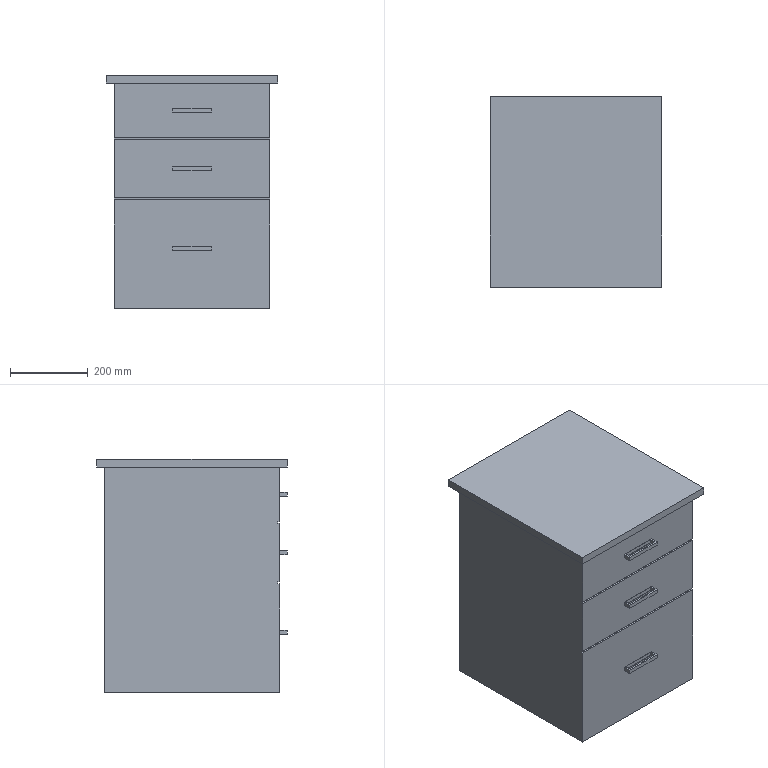Part | SolidWorks | features ICE 7, Extrusion 1 | 1 solid | 46 faces | box 440 x 490 x 600 mm | volume 108712401 mm3 | plane 46
STEP:
#1=CARTESIAN_POINT('',(400.,0.,280.));
#2=VERTEX_POINT('',#1);
#3=CARTESIAN_POINT('',(400.,0.,0.));
#4=VERTEX_POINT('',#3);
#5=CARTESIAN_POINT('',(400.,0.,600.));
#6=DIRECTION('',(0.,0.,-1.));
#7=VECTOR('',#6,1000.);
#8=LINE('',#5,#7);
#9=EDGE_CURVE('',#2,#4,#8,.T.);
#10=ORIENTED_EDGE('',*,*,#9,.F.);
#11=CARTESIAN_POINT('',(0.,0.,280.));
#12=VERTEX_POINT('',#11);
#13=CARTESIAN_POINT('',(0.,0.,280.));
#14=DIRECTION('',(1.,0.,0.));
#15=VECTOR('',#14,1000.);
#16=LINE('',#13,#15);
#17=EDGE_CURVE('',#12,#2,#16,.T.);
#18=ORIENTED_EDGE('',*,*,#17,.F.);
#19=CARTESIAN_POINT('',(0.,0.,0.));
#20=VERTEX_POINT('',#19);
#21=CARTESIAN_POINT('',(0.,0.,600.));
#22=DIRECTION('',(0.,0.,-1.));
#23=VECTOR('',#22,1000.);
#24=LINE('',#21,#23);
#25=EDGE_CURVE('',#12,#20,#24,.T.);
#26=ORIENTED_EDGE('',*,*,#25,.T.);
#27=CARTESIAN_POINT('',(0.,0.,0.));
#28=DIRECTION('',(1.,0.,0.));
#29=VECTOR('',#28,1000.);
#30=LINE('',#27,#29);
#31=EDGE_CURVE('',#20,#4,#30,.T.);
#32=ORIENTED_EDGE('',*,*,#31,.T.);
#33=EDGE_LOOP('',(#10,#18,#26,#32));
#34=FACE_OUTER_BOUND('',#33,.T.);
#35=CARTESIAN_POINT('',(150.,0.,160.));
#36=VERTEX_POINT('',#35);
#37=CARTESIAN_POINT('',(150.,0.,150.));
#38=VERTEX_POINT('',#37);
#39=CARTESIAN_POINT('',(150.,0.,150.));
#40=DIRECTION('',(0.,0.,-1.));
#41=VECTOR('',#40,1000.);
#42=LINE('',#39,#41);
#43=EDGE_CURVE('',#36,#38,#42,.T.);
#44=ORIENTED_EDGE('',*,*,#43,.F.);
#45=CARTESIAN_POINT('',(250.,0.,160.));
#46=VERTEX_POINT('',#45);
#47=CARTESIAN_POINT('',(150.,0.,160.));
#48=DIRECTION('',(-1.,0.,0.));
#49=VECTOR('',#48,1000.);
#50=LINE('',#47,#49);
#51=EDGE_CURVE('',#46,#36,#50,.T.);
#52=ORIENTED_EDGE('',*,*,#51,.F.);
#53=CARTESIAN_POINT('',(250.,0.,150.));
#54=VERTEX_POINT('',#53);
#55=CARTESIAN_POINT('',(250.,0.,150.));
#56=DIRECTION('',(0.,0.,1.));
#57=VECTOR('',#56,1000.);
#58=LINE('',#55,#57);
#59=EDGE_CURVE('',#54,#46,#58,.T.);
#60=ORIENTED_EDGE('',*,*,#59,.F.);
#61=CARTESIAN_POINT('',(150.,0.,150.));
#62=DIRECTION('',(1.,0.,0.));
#63=VECTOR('',#62,1000.);
#64=LINE('',#61,#63);
#65=EDGE_CURVE('',#38,#54,#64,.T.);
#66=ORIENTED_EDGE('',*,*,#65,.F.);
#67=EDGE_LOOP('',(#44,#52,#60,#66));
#68=FACE_BOUND('',#67,.T.);
#69=CARTESIAN_POINT('',(0.,0.,600.));
#70=DIRECTION('',(0.,1.,0.));
#71=DIRECTION('',(0.,0.,1.));
#72=AXIS2_PLACEMENT_3D('',#69,#70,#71);
#73=PLANE('',#72);
#74=ADVANCED_FACE('',(#34,#68),#73,.F.);
#75=CARTESIAN_POINT('',(0.,0.,435.));
#76=VERTEX_POINT('',#75);
#77=CARTESIAN_POINT('',(0.,0.,285.));
#78=VERTEX_POINT('',#77);
#79=CARTESIAN_POINT('',(0.,0.,600.));
#80=DIRECTION('',(0.,0.,-1.));
#81=VECTOR('',#80,1000.);
#82=LINE('',#79,#81);
#83=EDGE_CURVE('',#76,#78,#82,.T.);
#84=ORIENTED_EDGE('',*,*,#83,.T.);
#85=CARTESIAN_POINT('',(400.,0.,285.));
#86=VERTEX_POINT('',#85);
#87=CARTESIAN_POINT('',(0.,0.,285.));
#88=DIRECTION('',(-1.,0.,0.));
#89=VECTOR('',#88,1000.);
#90=LINE('',#87,#89);
#91=EDGE_CURVE('',#86,#78,#90,.T.);
#92=ORIENTED_EDGE('',*,*,#91,.F.);
#93=CARTESIAN_POINT('',(400.,0.,435.));
#94=VERTEX_POINT('',#93);
#95=CARTESIAN_POINT('',(400.,0.,600.));
#96=DIRECTION('',(0.,0.,-1.));
#97=VECTOR('',#96,1000.);
#98=LINE('',#95,#97);
#99=EDGE_CURVE('',#94,#86,#98,.T.);
#100=ORIENTED_EDGE('',*,*,#99,.F.);
#101=CARTESIAN_POINT('',(0.,0.,435.));
#102=DIRECTION('',(1.,0.,0.));
#103=VECTOR('',#102,1000.);
#104=LINE('',#101,#103);
#105=EDGE_CURVE('',#76,#94,#104,.T.);
#106=ORIENTED_EDGE('',*,*,#105,.F.);
#107=EDGE_LOOP('',(#84,#92,#100,#106));
#108=FACE_OUTER_BOUND('',#107,.T.);
#109=CARTESIAN_POINT('',(150.,0.,365.));
#110=VERTEX_POINT('',#109);
#111=CARTESIAN_POINT('',(150.,0.,355.));
#112=VERTEX_POINT('',#111);
#113=CARTESIAN_POINT('',(150.,0.,365.));
#114=DIRECTION('',(0.,0.,-1.));
#115=VECTOR('',#114,1000.);
#116=LINE('',#113,#115);
#117=EDGE_CURVE('',#110,#112,#116,.T.);
#118=ORIENTED_EDGE('',*,*,#117,.F.);
#119=CARTESIAN_POINT('',(250.,0.,365.));
#120=VERTEX_POINT('',#119);
#121=CARTESIAN_POINT('',(150.,0.,365.));
#122=DIRECTION('',(-1.,0.,0.));
#123=VECTOR('',#122,1000.);
#124=LINE('',#121,#123);
#125=EDGE_CURVE('',#120,#110,#124,.T.);
#126=ORIENTED_EDGE('',*,*,#125,.F.);
#127=CARTESIAN_POINT('',(250.,0.,355.));
#128=VERTEX_POINT('',#127);
#129=CARTESIAN_POINT('',(250.,0.,365.));
#130=DIRECTION('',(0.,0.,1.));
#131=VECTOR('',#130,1000.);
#132=LINE('',#129,#131);
#133=EDGE_CURVE('',#128,#120,#132,.T.);
#134=ORIENTED_EDGE('',*,*,#133,.F.);
#135=CARTESIAN_POINT('',(150.,0.,355.));
#136=DIRECTION('',(1.,0.,0.));
#137=VECTOR('',#136,1000.);
#138=LINE('',#135,#137);
#139=EDGE_CURVE('',#112,#128,#138,.T.);
#140=ORIENTED_EDGE('',*,*,#139,.F.);
#141=EDGE_LOOP('',(#118,#126,#134,#140));
#142=FACE_BOUND('',#141,.T.);
#143=CARTESIAN_POINT('',(0.,0.,600.));
#144=DIRECTION('',(0.,1.,0.));
#145=DIRECTION('',(0.,0.,1.));
#146=AXIS2_PLACEMENT_3D('',#143,#144,#145);
#147=PLANE('',#146);
#148=ADVANCED_FACE('',(#108,#142),#147,.F.);
#149=CARTESIAN_POINT('',(0.,0.,580.));
#150=VERTEX_POINT('',#149);
#151=CARTESIAN_POINT('',(0.,0.,440.));
#152=VERTEX_POINT('',#151);
#153=CARTESIAN_POINT('',(0.,0.,600.));
#154=DIRECTION('',(0.,0.,-1.));
#155=VECTOR('',#154,1000.);
#156=LINE('',#153,#155);
#157=EDGE_CURVE('',#150,#152,#156,.T.);
#158=ORIENTED_EDGE('',*,*,#157,.T.);
#159=CARTESIAN_POINT('',(400.,0.,440.));
#160=VERTEX_POINT('',#159);
#161=CARTESIAN_POINT('',(0.,0.,440.));
#162=DIRECTION('',(-1.,0.,0.));
#163=VECTOR('',#162,1000.);
#164=LINE('',#161,#163);
#165=EDGE_CURVE('',#160,#152,#164,.T.);
#166=ORIENTED_EDGE('',*,*,#165,.F.);
#167=CARTESIAN_POINT('',(400.,0.,580.));
#168=VERTEX_POINT('',#167);
#169=CARTESIAN_POINT('',(400.,0.,600.));
#170=DIRECTION('',(0.,0.,-1.));
#171=VECTOR('',#170,1000.);
#172=LINE('',#169,#171);
#173=EDGE_CURVE('',#168,#160,#172,.T.);
#174=ORIENTED_EDGE('',*,*,#173,.F.);
#175=CARTESIAN_POINT('',(0.,0.,580.));
#176=DIRECTION('',(1.,0.,0.));
#177=VECTOR('',#176,1000.);
#178=LINE('',#175,#177);
#179=EDGE_CURVE('',#150,#168,#178,.T.);
#180=ORIENTED_EDGE('',*,*,#179,.F.);
#181=EDGE_LOOP('',(#158,#166,#174,#180));
#182=FACE_OUTER_BOUND('',#181,.T.);
#183=CARTESIAN_POINT('',(150.,0.,515.));
#184=VERTEX_POINT('',#183);
#185=CARTESIAN_POINT('',(150.,0.,505.));
#186=VERTEX_POINT('',#185);
#187=CARTESIAN_POINT('',(150.,0.,515.));
#188=DIRECTION('',(0.,0.,-1.));
#189=VECTOR('',#188,1000.);
#190=LINE('',#187,#189);
#191=EDGE_CURVE('',#184,#186,#190,.T.);
#192=ORIENTED_EDGE('',*,*,#191,.F.);
#193=CARTESIAN_POINT('',(250.,0.,515.));
#194=VERTEX_POINT('',#193);
#195=CARTESIAN_POINT('',(150.,0.,515.));
#196=DIRECTION('',(-1.,0.,0.));
#197=VECTOR('',#196,1000.);
#198=LINE('',#195,#197);
#199=EDGE_CURVE('',#194,#184,#198,.T.);
#200=ORIENTED_EDGE('',*,*,#199,.F.);
#201=CARTESIAN_POINT('',(250.,0.,505.));
#202=VERTEX_POINT('',#201);
#203=CARTESIAN_POINT('',(250.,0.,515.));
#204=DIRECTION('',(0.,0.,1.));
#205=VECTOR('',#204,1000.);
#206=LINE('',#203,#205);
#207=EDGE_CURVE('',#202,#194,#206,.T.);
#208=ORIENTED_EDGE('',*,*,#207,.F.);
#209=CARTESIAN_POINT('',(150.,0.,505.));
#210=DIRECTION('',(1.,0.,0.));
#211=VECTOR('',#210,1000.);
#212=LINE('',#209,#211);
#213=EDGE_CURVE('',#186,#202,#212,.T.);
#214=ORIENTED_EDGE('',*,*,#213,.F.);
#215=EDGE_LOOP('',(#192,#200,#208,#214));
#216=FACE_BOUND('',#215,.T.);
#217=CARTESIAN_POINT('',(0.,0.,600.));
#218=DIRECTION('',(0.,1.,0.));
#219=DIRECTION('',(0.,0.,1.));
#220=AXIS2_PLACEMENT_3D('',#217,#218,#219);
#221=PLANE('',#220);
#222=ADVANCED_FACE('',(#182,#216),#221,.F.);
#223=CARTESIAN_POINT('',(0.,5.,285.));
#224=VERTEX_POINT('',#223);
#225=CARTESIAN_POINT('',(0.,5.,280.));
#226=VERTEX_POINT('',#225);
#227=CARTESIAN_POINT('',(0.,5.,285.));
#228=DIRECTION('',(0.,0.,-1.));
#229=VECTOR('',#228,1000.);
#230=LINE('',#227,#229);
#231=EDGE_CURVE('',#224,#226,#230,.T.);
#232=ORIENTED_EDGE('',*,*,#231,.F.);
#233=CARTESIAN_POINT('',(0.,5.,285.));
#234=DIRECTION('',(0.,-1.,0.));
#235=VECTOR('',#234,1000.);
#236=LINE('',#233,#235);
#237=EDGE_CURVE('',#224,#78,#236,.T.);
#238=ORIENTED_EDGE('',*,*,#237,.T.);
#239=ORIENTED_EDGE('',*,*,#83,.F.);
#240=CARTESIAN_POINT('',(0.,5.,435.));
#241=VERTEX_POINT('',#240);
#242=CARTESIAN_POINT('',(0.,5.,435.));
#243=DIRECTION('',(0.,-1.,0.));
#244=VECTOR('',#243,1000.);
#245=LINE('',#242,#244);
#246=EDGE_CURVE('',#241,#76,#245,.T.);
#247=ORIENTED_EDGE('',*,*,#246,.F.);
#248=CARTESIAN_POINT('',(0.,5.,440.));
#249=VERTEX_POINT('',#248);
#250=CARTESIAN_POINT('',(0.,5.,440.));
#251=DIRECTION('',(0.,0.,-1.));
#252=VECTOR('',#251,1000.);
#253=LINE('',#250,#252);
#254=EDGE_CURVE('',#249,#241,#253,.T.);
#255=ORIENTED_EDGE('',*,*,#254,.F.);
#256=CARTESIAN_POINT('',(0.,5.,440.));
#257=DIRECTION('',(0.,-1.,0.));
#258=VECTOR('',#257,1000.);
#259=LINE('',#256,#258);
#260=EDGE_CURVE('',#249,#152,#259,.T.);
#261=ORIENTED_EDGE('',*,*,#260,.T.);
#262=ORIENTED_EDGE('',*,*,#157,.F.);
#263=CARTESIAN_POINT('',(0.,450.,580.));
#264=VERTEX_POINT('',#263);
#265=CARTESIAN_POINT('',(0.,0.,580.));
#266=DIRECTION('',(0.,-1.,0.));
#267=VECTOR('',#266,1000.);
#268=LINE('',#265,#267);
#269=EDGE_CURVE('',#264,#150,#268,.T.);
#270=ORIENTED_EDGE('',*,*,#269,.F.);
#271=CARTESIAN_POINT('',(0.,450.,0.));
#272=VERTEX_POINT('',#271);
#273=CARTESIAN_POINT('',(0.,450.,600.));
#274=DIRECTION('',(0.,0.,-1.));
#275=VECTOR('',#274,1000.);
#276=LINE('',#273,#275);
#277=EDGE_CURVE('',#264,#272,#276,.T.);
#278=ORIENTED_EDGE('',*,*,#277,.T.);
#279=CARTESIAN_POINT('',(0.,0.,0.));
#280=DIRECTION('',(0.,-1.,0.));
#281=VECTOR('',#280,1000.);
#282=LINE('',#279,#281);
#283=EDGE_CURVE('',#272,#20,#282,.T.);
#284=ORIENTED_EDGE('',*,*,#283,.T.);
#285=ORIENTED_EDGE('',*,*,#25,.F.);
#286=CARTESIAN_POINT('',(0.,5.,280.));
#287=DIRECTION('',(0.,-1.,0.));
#288=VECTOR('',#287,1000.);
#289=LINE('',#286,#288);
#290=EDGE_CURVE('',#226,#12,#289,.T.);
#291=ORIENTED_EDGE('',*,*,#290,.F.);
#292=EDGE_LOOP('',(#232,#238,#239,#247,#255,#261,#262,#270,#278,#284,#285,#291));
#293=FACE_OUTER_BOUND('',#292,.T.);
#294=CARTESIAN_POINT('',(0.,0.,600.));
#295=DIRECTION('',(1.,0.,0.));
#296=DIRECTION('',(0.,0.,-1.));
#297=AXIS2_PLACEMENT_3D('',#294,#295,#296);
#298=PLANE('',#297);
#299=ADVANCED_FACE('',(#293),#298,.F.);
#300=ORIENTED_EDGE('',*,*,#99,.T.);
#301=CARTESIAN_POINT('',(400.,5.,285.));
#302=VERTEX_POINT('',#301);
#303=CARTESIAN_POINT('',(400.,5.,285.));
#304=DIRECTION('',(0.,-1.,0.));
#305=VECTOR('',#304,1000.);
#306=LINE('',#303,#305);
#307=EDGE_CURVE('',#302,#86,#306,.T.);
#308=ORIENTED_EDGE('',*,*,#307,.F.);
#309=CARTESIAN_POINT('',(400.,5.,280.));
#310=VERTEX_POINT('',#309);
#311=CARTESIAN_POINT('',(400.,5.,285.));
#312=DIRECTION('',(0.,0.,1.));
#313=VECTOR('',#312,1000.);
#314=LINE('',#311,#313);
#315=EDGE_CURVE('',#310,#302,#314,.T.);
#316=ORIENTED_EDGE('',*,*,#315,.F.);
#317=CARTESIAN_POINT('',(400.,5.,280.));
#318=DIRECTION('',(0.,-1.,0.));
#319=VECTOR('',#318,1000.);
#320=LINE('',#317,#319);
#321=EDGE_CURVE('',#310,#2,#320,.T.);
#322=ORIENTED_EDGE('',*,*,#321,.T.);
#323=ORIENTED_EDGE('',*,*,#9,.T.);
#324=CARTESIAN_POINT('',(400.,450.,0.));
#325=VERTEX_POINT('',#324);
#326=CARTESIAN_POINT('',(400.,0.,0.));
#327=DIRECTION('',(0.,1.,0.));
#328=VECTOR('',#327,1000.);
#329=LINE('',#326,#328);
#330=EDGE_CURVE('',#4,#325,#329,.T.);
#331=ORIENTED_EDGE('',*,*,#330,.T.);
#332=CARTESIAN_POINT('',(400.,450.,580.));
#333=VERTEX_POINT('',#332);
#334=CARTESIAN_POINT('',(400.,450.,600.));
#335=DIRECTION('',(0.,0.,-1.));
#336=VECTOR('',#335,1000.);
#337=LINE('',#334,#336);
#338=EDGE_CURVE('',#333,#325,#337,.T.);
#339=ORIENTED_EDGE('',*,*,#338,.F.);
#340=CARTESIAN_POINT('',(400.,0.,580.));
#341=DIRECTION('',(0.,1.,0.));
#342=VECTOR('',#341,1000.);
#343=LINE('',#340,#342);
#344=EDGE_CURVE('',#168,#333,#343,.T.);
#345=ORIENTED_EDGE('',*,*,#344,.F.);
#346=ORIENTED_EDGE('',*,*,#173,.T.);
#347=CARTESIAN_POINT('',(400.,5.,440.));
#348=VERTEX_POINT('',#347);
#349=CARTESIAN_POINT('',(400.,5.,440.));
#350=DIRECTION('',(0.,-1.,0.));
#351=VECTOR('',#350,1000.);
#352=LINE('',#349,#351);
#353=EDGE_CURVE('',#348,#160,#352,.T.);
#354=ORIENTED_EDGE('',*,*,#353,.F.);
#355=CARTESIAN_POINT('',(400.,5.,435.));
#356=VERTEX_POINT('',#355);
#357=CARTESIAN_POINT('',(400.,5.,440.));
#358=DIRECTION('',(0.,0.,1.));
#359=VECTOR('',#358,1000.);
#360=LINE('',#357,#359);
#361=EDGE_CURVE('',#356,#348,#360,.T.);
#362=ORIENTED_EDGE('',*,*,#361,.F.);
#363=CARTESIAN_POINT('',(400.,5.,435.));
#364=DIRECTION('',(0.,-1.,0.));
#365=VECTOR('',#364,1000.);
#366=LINE('',#363,#365);
#367=EDGE_CURVE('',#356,#94,#366,.T.);
#368=ORIENTED_EDGE('',*,*,#367,.T.);
#369=EDGE_LOOP('',(#300,#308,#316,#322,#323,#331,#339,#345,#346,#354,#362,#368));
#370=FACE_OUTER_BOUND('',#369,.T.);
#371=CARTESIAN_POINT('',(400.,0.,600.));
#372=DIRECTION('',(-1.,0.,0.));
#373=DIRECTION('',(0.,0.,1.));
#374=AXIS2_PLACEMENT_3D('',#371,#372,#373);
#375=PLANE('',#374);
#376=ADVANCED_FACE('',(#370),#375,.F.);
#377=CARTESIAN_POINT('',(0.,450.,580.));
#378=DIRECTION('',(-1.,0.,0.));
#379=VECTOR('',#378,1000.);
#380=LINE('',#377,#379);
#381=EDGE_CURVE('',#333,#264,#380,.T.);
#382=ORIENTED_EDGE('',*,*,#381,.F.);
#383=ORIENTED_EDGE('',*,*,#338,.T.);
#384=CARTESIAN_POINT('',(0.,450.,0.));
#385=DIRECTION('',(-1.,0.,0.));
#386=VECTOR('',#385,1000.);
#387=LINE('',#384,#386);
#388=EDGE_CURVE('',#325,#272,#387,.T.);
#389=ORIENTED_EDGE('',*,*,#388,.T.);
#390=ORIENTED_EDGE('',*,*,#277,.F.);
#391=EDGE_LOOP('',(#382,#383,#389,#390));
#392=FACE_OUTER_BOUND('',#391,.T.);
#393=CARTESIAN_POINT('',(0.,450.,600.));
#394=DIRECTION('',(0.,-1.,0.));
#395=DIRECTION('',(0.,0.,-1.));
#396=AXIS2_PLACEMENT_3D('',#393,#394,#395);
#397=PLANE('',#396);
#398=ADVANCED_FACE('',(#392),#397,.F.);
#399=ORIENTED_EDGE('',*,*,#283,.F.);
#400=ORIENTED_EDGE('',*,*,#388,.F.);
#401=ORIENTED_EDGE('',*,*,#330,.F.);
#402=ORIENTED_EDGE('',*,*,#31,.F.);
#403=EDGE_LOOP('',(#399,#400,#401,#402));
#404=FACE_OUTER_BOUND('',#403,.T.);
#405=CARTESIAN_POINT('',(0.,450.,0.));
#406=DIRECTION('',(0.,0.,-1.));
#407=DIRECTION('',(-1.,0.,0.));
#408=AXIS2_PLACEMENT_3D('',#405,#406,#407);
#409=PLANE('',#408);
#410=ADVANCED_FACE('',(#404),#409,.T.);
#411=CARTESIAN_POINT('',(-20.,470.,580.));
#412=VERTEX_POINT('',#411);
#413=CARTESIAN_POINT('',(-20.,-20.,580.));
#414=VERTEX_POINT('',#413);
#415=CARTESIAN_POINT('',(-20.,470.,580.));
#416=DIRECTION('',(0.,-1.,0.));
#417=VECTOR('',#416,1000.);
#418=LINE('',#415,#417);
#419=EDGE_CURVE('',#412,#414,#418,.T.);
#420=ORIENTED_EDGE('',*,*,#419,.F.);
#421=CARTESIAN_POINT('',(420.,470.,580.));
#422=VERTEX_POINT('',#421);
#423=CARTESIAN_POINT('',(-20.,470.,580.));
#424=DIRECTION('',(-1.,0.,0.));
#425=VECTOR('',#424,1000.);
#426=LINE('',#423,#425);
#427=EDGE_CURVE('',#422,#412,#426,.T.);
#428=ORIENTED_EDGE('',*,*,#427,.F.);
#429=CARTESIAN_POINT('',(420.,-20.,580.));
#430=VERTEX_POINT('',#429);
#431=CARTESIAN_POINT('',(420.,470.,580.));
#432=DIRECTION('',(0.,1.,0.));
#433=VECTOR('',#432,1000.);
#434=LINE('',#431,#433);
#435=EDGE_CURVE('',#430,#422,#434,.T.);
#436=ORIENTED_EDGE('',*,*,#435,.F.);
#437=CARTESIAN_POINT('',(-20.,-20.,580.));
#438=DIRECTION('',(1.,0.,0.));
#439=VECTOR('',#438,1000.);
#440=LINE('',#437,#439);
#441=EDGE_CURVE('',#414,#430,#440,.T.);
#442=ORIENTED_EDGE('',*,*,#441,.F.);
#443=EDGE_LOOP('',(#420,#428,#436,#442));
#444=FACE_OUTER_BOUND('',#443,.T.);
#445=ORIENTED_EDGE('',*,*,#381,.T.);
#446=ORIENTED_EDGE('',*,*,#269,.T.);
#447=ORIENTED_EDGE('',*,*,#179,.T.);
#448=ORIENTED_EDGE('',*,*,#344,.T.);
#449=EDGE_LOOP('',(#445,#446,#447,#448));
#450=FACE_BOUND('',#449,.T.);
#451=CARTESIAN_POINT('',(-20.,-20.,580.));
#452=DIRECTION('',(0.,0.,1.));
#453=DIRECTION('',(1.,0.,0.));
#454=AXIS2_PLACEMENT_3D('',#451,#452,#453);
#455=PLANE('',#454);
#456=ADVANCED_FACE('',(#444,#450),#455,.F.);
#457=CARTESIAN_POINT('',(-20.,470.,600.));
#458=VERTEX_POINT('',#457);
#459=CARTESIAN_POINT('',(-20.,-20.,600.));
#460=VERTEX_POINT('',#459);
#461=CARTESIAN_POINT('',(-20.,470.,600.));
#462=DIRECTION('',(0.,-1.,0.));
#463=VECTOR('',#462,1000.);
#464=LINE('',#461,#463);
#465=EDGE_CURVE('',#458,#460,#464,.T.);
#466=ORIENTED_EDGE('',*,*,#465,.F.);
#467=CARTESIAN_POINT('',(-20.,470.,580.));
#468=DIRECTION('',(0.,0.,1.));
#469=VECTOR('',#468,1000.);
#470=LINE('',#467,#469);
#471=EDGE_CURVE('',#412,#458,#470,.T.);
#472=ORIENTED_EDGE('',*,*,#471,.F.);
#473=ORIENTED_EDGE('',*,*,#419,.T.);
#474=CARTESIAN_POINT('',(-20.,-20.,580.));
#475=DIRECTION('',(0.,0.,1.));
#476=VECTOR('',#475,1000.);
#477=LINE('',#474,#476);
#478=EDGE_CURVE('',#414,#460,#477,.T.);
#479=ORIENTED_EDGE('',*,*,#478,.T.);
#480=EDGE_LOOP('',(#466,#472,#473,#479));
#481=FACE_OUTER_BOUND('',#480,.T.);
#482=CARTESIAN_POINT('',(-20.,470.,580.));
#483=DIRECTION('',(-1.,0.,0.));
#484=DIRECTION('',(0.,-1.,0.));
#485=AXIS2_PLACEMENT_3D('',#482,#483,#484);
#486=PLANE('',#485);
#487=ADVANCED_FACE('',(#481),#486,.T.);
#488=CARTESIAN_POINT('',(420.,470.,600.));
#489=VERTEX_POINT('',#488);
#490=CARTESIAN_POINT('',(-20.,470.,600.));
#491=DIRECTION('',(-1.,0.,0.));
#492=VECTOR('',#491,1000.);
#493=LINE('',#490,#492);
#494=EDGE_CURVE('',#489,#458,#493,.T.);
#495=ORIENTED_EDGE('',*,*,#494,.F.);
#496=CARTESIAN_POINT('',(420.,470.,580.));
#497=DIRECTION('',(0.,0.,1.));
#498=VECTOR('',#497,1000.);
#499=LINE('',#496,#498);
#500=EDGE_CURVE('',#422,#489,#499,.T.);
#501=ORIENTED_EDGE('',*,*,#500,.F.);
#502=ORIENTED_EDGE('',*,*,#427,.T.);
#503=ORIENTED_EDGE('',*,*,#471,.T.);
#504=EDGE_LOOP('',(#495,#501,#502,#503));
#505=FACE_OUTER_BOUND('',#504,.T.);
#506=CARTESIAN_POINT('',(-20.,470.,580.));
#507=DIRECTION('',(0.,1.,0.));
#508=DIRECTION('',(0.,0.,1.));
#509=AXIS2_PLACEMENT_3D('',#506,#507,#508);
#510=PLANE('',#509);
#511=ADVANCED_FACE('',(#505),#510,.T.);
#512=CARTESIAN_POINT('',(420.,-20.,600.));
#513=VERTEX_POINT('',#512);
#514=CARTESIAN_POINT('',(420.,470.,600.));
#515=DIRECTION('',(0.,1.,0.));
#516=VECTOR('',#515,1000.);
#517=LINE('',#514,#516);
#518=EDGE_CURVE('',#513,#489,#517,.T.);
#519=ORIENTED_EDGE('',*,*,#518,.F.);
#520=CARTESIAN_POINT('',(420.,-20.,580.));
#521=DIRECTION('',(0.,0.,1.));
#522=VECTOR('',#521,1000.);
#523=LINE('',#520,#522);
#524=EDGE_CURVE('',#430,#513,#523,.T.);
#525=ORIENTED_EDGE('',*,*,#524,.F.);
#526=ORIENTED_EDGE('',*,*,#435,.T.);
#527=ORIENTED_EDGE('',*,*,#500,.T.);
#528=EDGE_LOOP('',(#519,#525,#526,#527));
#529=FACE_OUTER_BOUND('',#528,.T.);
#530=CARTESIAN_POINT('',(420.,470.,580.));
#531=DIRECTION('',(1.,0.,0.));
#532=DIRECTION('',(0.,1.,0.));
#533=AXIS2_PLACEMENT_3D('',#530,#531,#532);
#534=PLANE('',#533);
#535=ADVANCED_FACE('',(#529),#534,.T.);
#536=CARTESIAN_POINT('',(-20.,-20.,600.));
#537=DIRECTION('',(1.,0.,0.));
#538=VECTOR('',#537,1000.);
#539=LINE('',#536,#538);
#540=EDGE_CURVE('',#460,#513,#539,.T.);
#541=ORIENTED_EDGE('',*,*,#540,.F.);
#542=ORIENTED_EDGE('',*,*,#478,.F.);
#543=ORIENTED_EDGE('',*,*,#441,.T.);
#544=ORIENTED_EDGE('',*,*,#524,.T.);
#545=EDGE_LOOP('',(#541,#542,#543,#544));
#546=FACE_OUTER_BOUND('',#545,.T.);
#547=CARTESIAN_POINT('',(-20.,-20.,580.));
#548=DIRECTION('',(0.,-1.,0.));
#549=DIRECTION('',(0.,0.,-1.));
#550=AXIS2_PLACEMENT_3D('',#547,#548,#549);
#551=PLANE('',#550);
#552=ADVANCED_FACE('',(#546),#551,.T.);
#553=ORIENTED_EDGE('',*,*,#465,.T.);
#554=ORIENTED_EDGE('',*,*,#540,.T.);
#555=ORIENTED_EDGE('',*,*,#518,.T.);
#556=ORIENTED_EDGE('',*,*,#494,.T.);
#557=EDGE_LOOP('',(#553,#554,#555,#556));
#558=FACE_OUTER_BOUND('',#557,.T.);
#559=CARTESIAN_POINT('',(0.,450.,600.));
#560=DIRECTION('',(0.,0.,-1.));
#561=DIRECTION('',(-1.,0.,0.));
#562=AXIS2_PLACEMENT_3D('',#559,#560,#561);
#563=PLANE('',#562);
#564=ADVANCED_FACE('',(#558),#563,.F.);
#565=ORIENTED_EDGE('',*,*,#165,.T.);
#566=ORIENTED_EDGE('',*,*,#260,.F.);
#567=CARTESIAN_POINT('',(0.,5.,440.));
#568=DIRECTION('',(-1.,0.,0.));
#569=VECTOR('',#568,1000.);
#570=LINE('',#567,#569);
#571=EDGE_CURVE('',#348,#249,#570,.T.);
#572=ORIENTED_EDGE('',*,*,#571,.F.);
#573=ORIENTED_EDGE('',*,*,#353,.T.);
#574=EDGE_LOOP('',(#565,#566,#572,#573));
#575=FACE_OUTER_BOUND('',#574,.T.);
#576=CARTESIAN_POINT('',(0.,5.,440.));
#577=DIRECTION('',(0.,0.,1.));
#578=DIRECTION('',(1.,0.,0.));
#579=AXIS2_PLACEMENT_3D('',#576,#577,#578);
#580=PLANE('',#579);
#581=ADVANCED_FACE('',(#575),#580,.F.);
#582=ORIENTED_EDGE('',*,*,#105,.T.);
#583=ORIENTED_EDGE('',*,*,#367,.F.);
#584=CARTESIAN_POINT('',(0.,5.,435.));
#585=DIRECTION('',(1.,0.,0.));
#586=VECTOR('',#585,1000.);
#587=LINE('',#584,#586);
#588=EDGE_CURVE('',#241,#356,#587,.T.);
#589=ORIENTED_EDGE('',*,*,#588,.F.);
#590=ORIENTED_EDGE('',*,*,#246,.T.);
#591=EDGE_LOOP('',(#582,#583,#589,#590));
#592=FACE_OUTER_BOUND('',#591,.T.);
#593=CARTESIAN_POINT('',(0.,5.,435.));
#594=DIRECTION('',(0.,0.,-1.));
#595=DIRECTION('',(-1.,0.,0.));
#596=AXIS2_PLACEMENT_3D('',#593,#594,#595);
#597=PLANE('',#596);
#598=ADVANCED_FACE('',(#592),#597,.F.);
#599=ORIENTED_EDGE('',*,*,#254,.T.);
#600=ORIENTED_EDGE('',*,*,#588,.T.);
#601=ORIENTED_EDGE('',*,*,#361,.T.);
#602=ORIENTED_EDGE('',*,*,#571,.T.);
#603=EDGE_LOOP('',(#599,#600,#601,#602));
#604=FACE_OUTER_BOUND('',#603,.T.);
#605=CARTESIAN_POINT('',(0.,5.,435.));
#606=DIRECTION('',(0.,-1.,0.));
#607=DIRECTION('',(0.,0.,-1.));
#608=AXIS2_PLACEMENT_3D('',#605,#606,#607);
#609=PLANE('',#608);
#610=ADVANCED_FACE('',(#604),#609,.T.);
#611=ORIENTED_EDGE('',*,*,#91,.T.);
#612=ORIENTED_EDGE('',*,*,#237,.F.);
#613=CARTESIAN_POINT('',(0.,5.,285.));
#614=DIRECTION('',(-1.,0.,0.));
#615=VECTOR('',#614,1000.);
#616=LINE('',#613,#615);
#617=EDGE_CURVE('',#302,#224,#616,.T.);
#618=ORIENTED_EDGE('',*,*,#617,.F.);
#619=ORIENTED_EDGE('',*,*,#307,.T.);
#620=EDGE_LOOP('',(#611,#612,#618,#619));
#621=FACE_OUTER_BOUND('',#620,.T.);
#622=CARTESIAN_POINT('',(0.,5.,285.));
#623=DIRECTION('',(0.,0.,1.));
#624=DIRECTION('',(1.,0.,0.));
#625=AXIS2_PLACEMENT_3D('',#622,#623,#624);
#626=PLANE('',#625);
#627=ADVANCED_FACE('',(#621),#626,.F.);
#628=ORIENTED_EDGE('',*,*,#17,.T.);
#629=ORIENTED_EDGE('',*,*,#321,.F.);
#630=CARTESIAN_POINT('',(0.,5.,280.));
#631=DIRECTION('',(1.,0.,0.));
#632=VECTOR('',#631,1000.);
#633=LINE('',#630,#632);
#634=EDGE_CURVE('',#226,#310,#633,.T.);
#635=ORIENTED_EDGE('',*,*,#634,.F.);
#636=ORIENTED_EDGE('',*,*,#290,.T.);
#637=EDGE_LOOP('',(#628,#629,#635,#636));
#638=FACE_OUTER_BOUND('',#637,.T.);
#639=CARTESIAN_POINT('',(0.,5.,280.));
#640=DIRECTION('',(0.,0.,-1.));
#641=DIRECTION('',(-1.,0.,0.));
#642=AXIS2_PLACEMENT_3D('',#639,#640,#641);
#643=PLANE('',#642);
#644=ADVANCED_FACE('',(#638),#643,.F.);
#645=ORIENTED_EDGE('',*,*,#231,.T.);
#646=ORIENTED_EDGE('',*,*,#634,.T.);
#647=ORIENTED_EDGE('',*,*,#315,.T.);
#648=ORIENTED_EDGE('',*,*,#617,.T.);
#649=EDGE_LOOP('',(#645,#646,#647,#648));
#650=FACE_OUTER_BOUND('',#649,.T.);
#651=CARTESIAN_POINT('',(0.,5.,280.));
#652=DIRECTION('',(0.,-1.,0.));
#653=DIRECTION('',(0.,0.,-1.));
#654=AXIS2_PLACEMENT_3D('',#651,#652,#653);
#655=PLANE('',#654);
#656=ADVANCED_FACE('',(#650),#655,.T.);
#657=ORIENTED_EDGE('',*,*,#191,.T.);
#658=CARTESIAN_POINT('',(150.,-20.,505.));
#659=VERTEX_POINT('',#658);
#660=CARTESIAN_POINT('',(150.,-20.,505.));
#661=DIRECTION('',(0.,1.,0.));
#662=VECTOR('',#661,1000.);
#663=LINE('',#660,#662);
#664=EDGE_CURVE('',#659,#186,#663,.T.);
#665=ORIENTED_EDGE('',*,*,#664,.F.);
#666=CARTESIAN_POINT('',(150.,-20.,515.));
#667=VERTEX_POINT('',#666);
#668=CARTESIAN_POINT('',(150.,-20.,515.));
#669=DIRECTION('',(0.,0.,-1.));
#670=VECTOR('',#669,1000.);
#671=LINE('',#668,#670);
#672=EDGE_CURVE('',#667,#659,#671,.T.);
#673=ORIENTED_EDGE('',*,*,#672,.F.);
#674=CARTESIAN_POINT('',(150.,-20.,515.));
#675=DIRECTION('',(0.,1.,0.));
#676=VECTOR('',#675,1000.);
#677=LINE('',#674,#676);
#678=EDGE_CURVE('',#667,#184,#677,.T.);
#679=ORIENTED_EDGE('',*,*,#678,.T.);
#680=EDGE_LOOP('',(#657,#665,#673,#679));
#681=FACE_OUTER_BOUND('',#680,.T.);
#682=CARTESIAN_POINT('',(150.,-20.,515.));
#683=DIRECTION('',(1.,0.,0.));
#684=DIRECTION('',(0.,0.,-1.));
#685=AXIS2_PLACEMENT_3D('',#682,#683,#684);
#686=PLANE('',#685);
#687=ADVANCED_FACE('',(#681),#686,.F.);
#688=CARTESIAN_POINT('',(245.,-0.3339,505.));
#689=VERTEX_POINT('',#688);
#690=CARTESIAN_POINT('',(155.,-0.3339,505.));
#691=VERTEX_POINT('',#690);
#692=CARTESIAN_POINT('',(150.,-0.3339,505.));
#693=DIRECTION('',(-1.,0.,0.));
#694=VECTOR('',#693,1000.);
#695=LINE('',#692,#694);
#696=EDGE_CURVE('',#689,#691,#695,.T.);
#697=ORIENTED_EDGE('',*,*,#696,.T.);
#698=CARTESIAN_POINT('',(155.,-15.,505.));
#699=VERTEX_POINT('',#698);
#700=CARTESIAN_POINT('',(155.,-20.,505.));
#701=DIRECTION('',(0.,-1.,0.));
#702=VECTOR('',#701,1000.);
#703=LINE('',#700,#702);
#704=EDGE_CURVE('',#691,#699,#703,.T.);
#705=ORIENTED_EDGE('',*,*,#704,.T.);
#706=CARTESIAN_POINT('',(245.,-15.,505.));
#707=VERTEX_POINT('',#706);
#708=CARTESIAN_POINT('',(150.,-15.,505.));
#709=DIRECTION('',(1.,0.,0.));
#710=VECTOR('',#709,1000.);
#711=LINE('',#708,#710);
#712=EDGE_CURVE('',#699,#707,#711,.T.);
#713=ORIENTED_EDGE('',*,*,#712,.T.);
#714=CARTESIAN_POINT('',(245.,-20.,505.));
#715=DIRECTION('',(0.,1.,0.));
#716=VECTOR('',#715,1000.);
#717=LINE('',#714,#716);
#718=EDGE_CURVE('',#707,#689,#717,.T.);
#719=ORIENTED_EDGE('',*,*,#718,.T.);
#720=EDGE_LOOP('',(#697,#705,#713,#719));
#721=FACE_BOUND('',#720,.T.);
#722=ORIENTED_EDGE('',*,*,#213,.T.);
#723=CARTESIAN_POINT('',(250.,-20.,505.));
#724=VERTEX_POINT('',#723);
#725=CARTESIAN_POINT('',(250.,-20.,505.));
#726=DIRECTION('',(0.,1.,0.));
#727=VECTOR('',#726,1000.);
#728=LINE('',#725,#727);
#729=EDGE_CURVE('',#724,#202,#728,.T.);
#730=ORIENTED_EDGE('',*,*,#729,.F.);
#731=CARTESIAN_POINT('',(150.,-20.,505.));
#732=DIRECTION('',(1.,0.,0.));
#733=VECTOR('',#732,1000.);
#734=LINE('',#731,#733);
#735=EDGE_CURVE('',#659,#724,#734,.T.);
#736=ORIENTED_EDGE('',*,*,#735,.F.);
#737=ORIENTED_EDGE('',*,*,#664,.T.);
#738=EDGE_LOOP('',(#722,#730,#736,#737));
#739=FACE_OUTER_BOUND('',#738,.T.);
#740=CARTESIAN_POINT('',(150.,-20.,505.));
#741=DIRECTION('',(0.,0.,1.));
#742=DIRECTION('',(1.,0.,0.));
#743=AXIS2_PLACEMENT_3D('',#740,#741,#742);
#744=PLANE('',#743);
#745=ADVANCED_FACE('',(#721,#739),#744,.F.);
#746=ORIENTED_EDGE('',*,*,#207,.T.);
#747=CARTESIAN_POINT('',(250.,-20.,515.));
#748=VERTEX_POINT('',#747);
#749=CARTESIAN_POINT('',(250.,-20.,515.));
#750=DIRECTION('',(0.,1.,0.));
#751=VECTOR('',#750,1000.);
#752=LINE('',#749,#751);
#753=EDGE_CURVE('',#748,#194,#752,.T.);
#754=ORIENTED_EDGE('',*,*,#753,.F.);
#755=CARTESIAN_POINT('',(250.,-20.,515.));
#756=DIRECTION('',(0.,0.,1.));
#757=VECTOR('',#756,1000.);
#758=LINE('',#755,#757);
#759=EDGE_CURVE('',#724,#748,#758,.T.);
#760=ORIENTED_EDGE('',*,*,#759,.F.);
#761=ORIENTED_EDGE('',*,*,#729,.T.);
#762=EDGE_LOOP('',(#746,#754,#760,#761));
#763=FACE_OUTER_BOUND('',#762,.T.);
#764=CARTESIAN_POINT('',(250.,-20.,515.));
#765=DIRECTION('',(-1.,0.,0.));
#766=DIRECTION('',(0.,0.,1.));
#767=AXIS2_PLACEMENT_3D('',#764,#765,#766);
#768=PLANE('',#767);
#769=ADVANCED_FACE('',(#763),#768,.F.);
#770=CARTESIAN_POINT('',(155.,-15.,515.));
#771=VERTEX_POINT('',#770);
#772=CARTESIAN_POINT('',(245.,-15.,515.));
#773=VERTEX_POINT('',#772);
#774=CARTESIAN_POINT('',(155.,-15.,515.));
#775=DIRECTION('',(1.,0.,0.));
#776=VECTOR('',#775,1000.);
#777=LINE('',#774,#776);
#778=EDGE_CURVE('',#771,#773,#777,.T.);
#779=ORIENTED_EDGE('',*,*,#778,.F.);
#780=CARTESIAN_POINT('',(155.,-0.3339,515.));
#781=VERTEX_POINT('',#780);
#782=CARTESIAN_POINT('',(155.,-0.3339,515.));
#783=DIRECTION('',(0.,-1.,0.));
#784=VECTOR('',#783,1000.);
#785=LINE('',#782,#784);
#786=EDGE_CURVE('',#781,#771,#785,.T.);
#787=ORIENTED_EDGE('',*,*,#786,.F.);
#788=CARTESIAN_POINT('',(245.,-0.3339,515.));
#789=VERTEX_POINT('',#788);
#790=CARTESIAN_POINT('',(155.,-0.3339,515.));
#791=DIRECTION('',(-1.,0.,0.));
#792=VECTOR('',#791,1000.);
#793=LINE('',#790,#792);
#794=EDGE_CURVE('',#789,#781,#793,.T.);
#795=ORIENTED_EDGE('',*,*,#794,.F.);
#796=CARTESIAN_POINT('',(245.,-0.3339,515.));
#797=DIRECTION('',(0.,1.,0.));
#798=VECTOR('',#797,1000.);
#799=LINE('',#796,#798);
#800=EDGE_CURVE('',#773,#789,#799,.T.);
#801=ORIENTED_EDGE('',*,*,#800,.F.);
#802=EDGE_LOOP('',(#779,#787,#795,#801));
#803=FACE_BOUND('',#802,.T.);
#804=ORIENTED_EDGE('',*,*,#199,.T.);
#805=ORIENTED_EDGE('',*,*,#678,.F.);
#806=CARTESIAN_POINT('',(150.,-20.,515.));
#807=DIRECTION('',(-1.,0.,0.));
#808=VECTOR('',#807,1000.);
#809=LINE('',#806,#808);
#810=EDGE_CURVE('',#748,#667,#809,.T.);
#811=ORIENTED_EDGE('',*,*,#810,.F.);
#812=ORIENTED_EDGE('',*,*,#753,.T.);
#813=EDGE_LOOP('',(#804,#805,#811,#812));
#814=FACE_OUTER_BOUND('',#813,.T.);
#815=CARTESIAN_POINT('',(150.,-20.,515.));
#816=DIRECTION('',(0.,0.,-1.));
#817=DIRECTION('',(-1.,0.,0.));
#818=AXIS2_PLACEMENT_3D('',#815,#816,#817);
#819=PLANE('',#818);
#820=ADVANCED_FACE('',(#803,#814),#819,.F.);
#821=ORIENTED_EDGE('',*,*,#672,.T.);
#822=ORIENTED_EDGE('',*,*,#735,.T.);
#823=ORIENTED_EDGE('',*,*,#759,.T.);
#824=ORIENTED_EDGE('',*,*,#810,.T.);
#825=EDGE_LOOP('',(#821,#822,#823,#824));
#826=FACE_OUTER_BOUND('',#825,.T.);
#827=CARTESIAN_POINT('',(150.,-20.,505.));
#828=DIRECTION('',(0.,-1.,0.));
#829=DIRECTION('',(0.,0.,-1.));
#830=AXIS2_PLACEMENT_3D('',#827,#828,#829);
#831=PLANE('',#830);
#832=ADVANCED_FACE('',(#826),#831,.T.);
#833=ORIENTED_EDGE('',*,*,#117,.T.);
#834=CARTESIAN_POINT('',(150.,-20.,355.));
#835=VERTEX_POINT('',#834);
#836=CARTESIAN_POINT('',(150.,-20.,355.));
#837=DIRECTION('',(0.,1.,0.));
#838=VECTOR('',#837,1000.);
#839=LINE('',#836,#838);
#840=EDGE_CURVE('',#835,#112,#839,.T.);
#841=ORIENTED_EDGE('',*,*,#840,.F.);
#842=CARTESIAN_POINT('',(150.,-20.,365.));
#843=VERTEX_POINT('',#842);
#844=CARTESIAN_POINT('',(150.,-20.,365.));
#845=DIRECTION('',(0.,0.,-1.));
#846=VECTOR('',#845,1000.);
#847=LINE('',#844,#846);
#848=EDGE_CURVE('',#843,#835,#847,.T.);
#849=ORIENTED_EDGE('',*,*,#848,.F.);
#850=CARTESIAN_POINT('',(150.,-20.,365.));
#851=DIRECTION('',(0.,1.,0.));
#852=VECTOR('',#851,1000.);
#853=LINE('',#850,#852);
#854=EDGE_CURVE('',#843,#110,#853,.T.);
#855=ORIENTED_EDGE('',*,*,#854,.T.);
#856=EDGE_LOOP('',(#833,#841,#849,#855));
#857=FACE_OUTER_BOUND('',#856,.T.);
#858=CARTESIAN_POINT('',(150.,-20.,365.));
#859=DIRECTION('',(1.,0.,0.));
#860=DIRECTION('',(0.,0.,-1.));
#861=AXIS2_PLACEMENT_3D('',#858,#859,#860);
#862=PLANE('',#861);
#863=ADVANCED_FACE('',(#857),#862,.F.);
#864=CARTESIAN_POINT('',(245.,-0.3339,355.));
#865=VERTEX_POINT('',#864);
#866=CARTESIAN_POINT('',(155.,-0.3339,355.));
#867=VERTEX_POINT('',#866);
#868=CARTESIAN_POINT('',(150.,-0.3339,355.));
#869=DIRECTION('',(-1.,0.,0.));
#870=VECTOR('',#869,1000.);
#871=LINE('',#868,#870);
#872=EDGE_CURVE('',#865,#867,#871,.T.);
#873=ORIENTED_EDGE('',*,*,#872,.T.);
#874=CARTESIAN_POINT('',(155.,-15.,355.));
#875=VERTEX_POINT('',#874);
#876=CARTESIAN_POINT('',(155.,-20.,355.));
#877=DIRECTION('',(0.,-1.,0.));
#878=VECTOR('',#877,1000.);
#879=LINE('',#876,#878);
#880=EDGE_CURVE('',#867,#875,#879,.T.);
#881=ORIENTED_EDGE('',*,*,#880,.T.);
#882=CARTESIAN_POINT('',(245.,-15.,355.));
#883=VERTEX_POINT('',#882);
#884=CARTESIAN_POINT('',(150.,-15.,355.));
#885=DIRECTION('',(1.,0.,0.));
#886=VECTOR('',#885,1000.);
#887=LINE('',#884,#886);
#888=EDGE_CURVE('',#875,#883,#887,.T.);
#889=ORIENTED_EDGE('',*,*,#888,.T.);
#890=CARTESIAN_POINT('',(245.,-20.,355.));
#891=DIRECTION('',(0.,1.,0.));
#892=VECTOR('',#891,1000.);
#893=LINE('',#890,#892);
#894=EDGE_CURVE('',#883,#865,#893,.T.);
#895=ORIENTED_EDGE('',*,*,#894,.T.);
#896=EDGE_LOOP('',(#873,#881,#889,#895));
#897=FACE_BOUND('',#896,.T.);
#898=ORIENTED_EDGE('',*,*,#139,.T.);
#899=CARTESIAN_POINT('',(250.,-20.,355.));
#900=VERTEX_POINT('',#899);
#901=CARTESIAN_POINT('',(250.,-20.,355.));
#902=DIRECTION('',(0.,1.,0.));
#903=VECTOR('',#902,1000.);
#904=LINE('',#901,#903);
#905=EDGE_CURVE('',#900,#128,#904,.T.);
#906=ORIENTED_EDGE('',*,*,#905,.F.);
#907=CARTESIAN_POINT('',(150.,-20.,355.));
#908=DIRECTION('',(1.,0.,0.));
#909=VECTOR('',#908,1000.);
#910=LINE('',#907,#909);
#911=EDGE_CURVE('',#835,#900,#910,.T.);
#912=ORIENTED_EDGE('',*,*,#911,.F.);
#913=ORIENTED_EDGE('',*,*,#840,.T.);
#914=EDGE_LOOP('',(#898,#906,#912,#913));
#915=FACE_OUTER_BOUND('',#914,.T.);
#916=CARTESIAN_POINT('',(150.,-20.,355.));
#917=DIRECTION('',(0.,0.,1.));
#918=DIRECTION('',(1.,0.,0.));
#919=AXIS2_PLACEMENT_3D('',#916,#917,#918);
#920=PLANE('',#919);
#921=ADVANCED_FACE('',(#897,#915),#920,.F.);
#922=ORIENTED_EDGE('',*,*,#133,.T.);
#923=CARTESIAN_POINT('',(250.,-20.,365.));
#924=VERTEX_POINT('',#923);
#925=CARTESIAN_POINT('',(250.,-20.,365.));
#926=DIRECTION('',(0.,1.,0.));
#927=VECTOR('',#926,1000.);
#928=LINE('',#925,#927);
#929=EDGE_CURVE('',#924,#120,#928,.T.);
#930=ORIENTED_EDGE('',*,*,#929,.F.);
#931=CARTESIAN_POINT('',(250.,-20.,365.));
#932=DIRECTION('',(0.,0.,1.));
#933=VECTOR('',#932,1000.);
#934=LINE('',#931,#933);
#935=EDGE_CURVE('',#900,#924,#934,.T.);
#936=ORIENTED_EDGE('',*,*,#935,.F.);
#937=ORIENTED_EDGE('',*,*,#905,.T.);
#938=EDGE_LOOP('',(#922,#930,#936,#937));
#939=FACE_OUTER_BOUND('',#938,.T.);
#940=CARTESIAN_POINT('',(250.,-20.,365.));
#941=DIRECTION('',(-1.,0.,0.));
#942=DIRECTION('',(0.,0.,1.));
#943=AXIS2_PLACEMENT_3D('',#940,#941,#942);
#944=PLANE('',#943);
#945=ADVANCED_FACE('',(#939),#944,.F.);
#946=CARTESIAN_POINT('',(245.,-15.,365.));
#947=VERTEX_POINT('',#946);
#948=CARTESIAN_POINT('',(155.,-15.,365.));
#949=VERTEX_POINT('',#948);
#950=CARTESIAN_POINT('',(150.,-15.,365.));
#951=DIRECTION('',(-1.,0.,0.));
#952=VECTOR('',#951,1000.);
#953=LINE('',#950,#952);
#954=EDGE_CURVE('',#947,#949,#953,.T.);
#955=ORIENTED_EDGE('',*,*,#954,.T.);
#956=CARTESIAN_POINT('',(155.,-0.3339,365.));
#957=VERTEX_POINT('',#956);
#958=CARTESIAN_POINT('',(155.,-20.,365.));
#959=DIRECTION('',(0.,1.,0.));
#960=VECTOR('',#959,1000.);
#961=LINE('',#958,#960);
#962=EDGE_CURVE('',#949,#957,#961,.T.);
#963=ORIENTED_EDGE('',*,*,#962,.T.);
#964=CARTESIAN_POINT('',(245.,-0.3339,365.));
#965=VERTEX_POINT('',#964);
#966=CARTESIAN_POINT('',(150.,-0.3339,365.));
#967=DIRECTION('',(1.,0.,0.));
#968=VECTOR('',#967,1000.);
#969=LINE('',#966,#968);
#970=EDGE_CURVE('',#957,#965,#969,.T.);
#971=ORIENTED_EDGE('',*,*,#970,.T.);
#972=CARTESIAN_POINT('',(245.,-20.,365.));
#973=DIRECTION('',(0.,-1.,0.));
#974=VECTOR('',#973,1000.);
#975=LINE('',#972,#974);
#976=EDGE_CURVE('',#965,#947,#975,.T.);
#977=ORIENTED_EDGE('',*,*,#976,.T.);
#978=EDGE_LOOP('',(#955,#963,#971,#977));
#979=FACE_BOUND('',#978,.T.);
#980=ORIENTED_EDGE('',*,*,#125,.T.);
#981=ORIENTED_EDGE('',*,*,#854,.F.);
#982=CARTESIAN_POINT('',(150.,-20.,365.));
#983=DIRECTION('',(-1.,0.,0.));
#984=VECTOR('',#983,1000.);
#985=LINE('',#982,#984);
#986=EDGE_CURVE('',#924,#843,#985,.T.);
#987=ORIENTED_EDGE('',*,*,#986,.F.);
#988=ORIENTED_EDGE('',*,*,#929,.T.);
#989=EDGE_LOOP('',(#980,#981,#987,#988));
#990=FACE_OUTER_BOUND('',#989,.T.);
#991=CARTESIAN_POINT('',(150.,-20.,365.));
#992=DIRECTION('',(0.,0.,-1.));
#993=DIRECTION('',(-1.,0.,0.));
#994=AXIS2_PLACEMENT_3D('',#991,#992,#993);
#995=PLANE('',#994);
#996=ADVANCED_FACE('',(#979,#990),#995,.F.);
#997=ORIENTED_EDGE('',*,*,#848,.T.);
#998=ORIENTED_EDGE('',*,*,#911,.T.);
#999=ORIENTED_EDGE('',*,*,#935,.T.);
#1000=ORIENTED_EDGE('',*,*,#986,.T.);
#1001=EDGE_LOOP('',(#997,#998,#999,#1000));
#1002=FACE_OUTER_BOUND('',#1001,.T.);
#1003=CARTESIAN_POINT('',(150.,-20.,355.));
#1004=DIRECTION('',(0.,-1.,0.));
#1005=DIRECTION('',(0.,0.,-1.));
#1006=AXIS2_PLACEMENT_3D('',#1003,#1004,#1005);
#1007=PLANE('',#1006);
#1008=ADVANCED_FACE('',(#1002),#1007,.T.);
#1009=ORIENTED_EDGE('',*,*,#43,.T.);
#1010=CARTESIAN_POINT('',(150.,-20.,150.));
#1011=VERTEX_POINT('',#1010);
#1012=CARTESIAN_POINT('',(150.,-20.,150.));
#1013=DIRECTION('',(0.,1.,0.));
#1014=VECTOR('',#1013,1000.);
#1015=LINE('',#1012,#1014);
#1016=EDGE_CURVE('',#1011,#38,#1015,.T.);
#1017=ORIENTED_EDGE('',*,*,#1016,.F.);
#1018=CARTESIAN_POINT('',(150.,-20.,160.));
#1019=VERTEX_POINT('',#1018);
#1020=CARTESIAN_POINT('',(150.,-20.,150.));
#1021=DIRECTION('',(0.,0.,-1.));
#1022=VECTOR('',#1021,1000.);
#1023=LINE('',#1020,#1022);
#1024=EDGE_CURVE('',#1019,#1011,#1023,.T.);
#1025=ORIENTED_EDGE('',*,*,#1024,.F.);
#1026=CARTESIAN_POINT('',(150.,-20.,160.));
#1027=DIRECTION('',(0.,1.,0.));
#1028=VECTOR('',#1027,1000.);
#1029=LINE('',#1026,#1028);
#1030=EDGE_CURVE('',#1019,#36,#1029,.T.);
#1031=ORIENTED_EDGE('',*,*,#1030,.T.);
#1032=EDGE_LOOP('',(#1009,#1017,#1025,#1031));
#1033=FACE_OUTER_BOUND('',#1032,.T.);
#1034=CARTESIAN_POINT('',(150.,-20.,150.));
#1035=DIRECTION('',(1.,0.,0.));
#1036=DIRECTION('',(0.,0.,-1.));
#1037=AXIS2_PLACEMENT_3D('',#1034,#1035,#1036);
#1038=PLANE('',#1037);
#1039=ADVANCED_FACE('',(#1033),#1038,.F.);
#1040=CARTESIAN_POINT('',(245.,-0.3339,150.));
#1041=VERTEX_POINT('',#1040);
#1042=CARTESIAN_POINT('',(155.,-0.3339,150.));
#1043=VERTEX_POINT('',#1042);
#1044=CARTESIAN_POINT('',(150.,-0.3339,150.));
#1045=DIRECTION('',(-1.,0.,0.));
#1046=VECTOR('',#1045,1000.);
#1047=LINE('',#1044,#1046);
#1048=EDGE_CURVE('',#1041,#1043,#1047,.T.);
#1049=ORIENTED_EDGE('',*,*,#1048,.T.);
#1050=CARTESIAN_POINT('',(155.,-15.,150.));
#1051=VERTEX_POINT('',#1050);
#1052=CARTESIAN_POINT('',(155.,-20.,150.));
#1053=DIRECTION('',(0.,-1.,0.));
#1054=VECTOR('',#1053,1000.);
#1055=LINE('',#1052,#1054);
#1056=EDGE_CURVE('',#1043,#1051,#1055,.T.);
#1057=ORIENTED_EDGE('',*,*,#1056,.T.);
#1058=CARTESIAN_POINT('',(245.,-15.,150.));
#1059=VERTEX_POINT('',#1058);
#1060=CARTESIAN_POINT('',(150.,-15.,150.));
#1061=DIRECTION('',(1.,0.,0.));
#1062=VECTOR('',#1061,1000.);
#1063=LINE('',#1060,#1062);
#1064=EDGE_CURVE('',#1051,#1059,#1063,.T.);
#1065=ORIENTED_EDGE('',*,*,#1064,.T.);
#1066=CARTESIAN_POINT('',(245.,-20.,150.));
#1067=DIRECTION('',(0.,1.,0.));
#1068=VECTOR('',#1067,1000.);
#1069=LINE('',#1066,#1068);
#1070=EDGE_CURVE('',#1059,#1041,#1069,.T.);
#1071=ORIENTED_EDGE('',*,*,#1070,.T.);
#1072=EDGE_LOOP('',(#1049,#1057,#1065,#1071));
#1073=FACE_BOUND('',#1072,.T.);
#1074=ORIENTED_EDGE('',*,*,#65,.T.);
#1075=CARTESIAN_POINT('',(250.,-20.,150.));
#1076=VERTEX_POINT('',#1075);
#1077=CARTESIAN_POINT('',(250.,-20.,150.));
#1078=DIRECTION('',(0.,1.,0.));
#1079=VECTOR('',#1078,1000.);
#1080=LINE('',#1077,#1079);
#1081=EDGE_CURVE('',#1076,#54,#1080,.T.);
#1082=ORIENTED_EDGE('',*,*,#1081,.F.);
#1083=CARTESIAN_POINT('',(150.,-20.,150.));
#1084=DIRECTION('',(1.,0.,0.));
#1085=VECTOR('',#1084,1000.);
#1086=LINE('',#1083,#1085);
#1087=EDGE_CURVE('',#1011,#1076,#1086,.T.);
#1088=ORIENTED_EDGE('',*,*,#1087,.F.);
#1089=ORIENTED_EDGE('',*,*,#1016,.T.);
#1090=EDGE_LOOP('',(#1074,#1082,#1088,#1089));
#1091=FACE_OUTER_BOUND('',#1090,.T.);
#1092=CARTESIAN_POINT('',(150.,-20.,150.));
#1093=DIRECTION('',(0.,0.,1.));
#1094=DIRECTION('',(1.,0.,0.));
#1095=AXIS2_PLACEMENT_3D('',#1092,#1093,#1094);
#1096=PLANE('',#1095);
#1097=ADVANCED_FACE('',(#1073,#1091),#1096,.F.);
#1098=ORIENTED_EDGE('',*,*,#59,.T.);
#1099=CARTESIAN_POINT('',(250.,-20.,160.));
#1100=VERTEX_POINT('',#1099);
#1101=CARTESIAN_POINT('',(250.,-20.,160.));
#1102=DIRECTION('',(0.,1.,0.));
#1103=VECTOR('',#1102,1000.);
#1104=LINE('',#1101,#1103);
#1105=EDGE_CURVE('',#1100,#46,#1104,.T.);
#1106=ORIENTED_EDGE('',*,*,#1105,.F.);
#1107=CARTESIAN_POINT('',(250.,-20.,150.));
#1108=DIRECTION('',(0.,0.,1.));
#1109=VECTOR('',#1108,1000.);
#1110=LINE('',#1107,#1109);
#1111=EDGE_CURVE('',#1076,#1100,#1110,.T.);
#1112=ORIENTED_EDGE('',*,*,#1111,.F.);
#1113=ORIENTED_EDGE('',*,*,#1081,.T.);
#1114=EDGE_LOOP('',(#1098,#1106,#1112,#1113));
#1115=FACE_OUTER_BOUND('',#1114,.T.);
#1116=CARTESIAN_POINT('',(250.,-20.,150.));
#1117=DIRECTION('',(-1.,0.,0.));
#1118=DIRECTION('',(0.,0.,1.));
#1119=AXIS2_PLACEMENT_3D('',#1116,#1117,#1118);
#1120=PLANE('',#1119);
#1121=ADVANCED_FACE('',(#1115),#1120,.F.);
#1122=CARTESIAN_POINT('',(245.,-15.,160.));
#1123=VERTEX_POINT('',#1122);
#1124=CARTESIAN_POINT('',(155.,-15.,160.));
#1125=VERTEX_POINT('',#1124);
#1126=CARTESIAN_POINT('',(150.,-15.,160.));
#1127=DIRECTION('',(-1.,0.,0.));
#1128=VECTOR('',#1127,1000.);
#1129=LINE('',#1126,#1128);
#1130=EDGE_CURVE('',#1123,#1125,#1129,.T.);
#1131=ORIENTED_EDGE('',*,*,#1130,.T.);
#1132=CARTESIAN_POINT('',(155.,-0.3339,160.));
#1133=VERTEX_POINT('',#1132);
#1134=CARTESIAN_POINT('',(155.,-20.,160.));
#1135=DIRECTION('',(0.,1.,0.));
#1136=VECTOR('',#1135,1000.);
#1137=LINE('',#1134,#1136);
#1138=EDGE_CURVE('',#1125,#1133,#1137,.T.);
#1139=ORIENTED_EDGE('',*,*,#1138,.T.);
#1140=CARTESIAN_POINT('',(245.,-0.3339,160.));
#1141=VERTEX_POINT('',#1140);
#1142=CARTESIAN_POINT('',(150.,-0.3339,160.));
#1143=DIRECTION('',(1.,0.,0.));
#1144=VECTOR('',#1143,1000.);
#1145=LINE('',#1142,#1144);
#1146=EDGE_CURVE('',#1133,#1141,#1145,.T.);
#1147=ORIENTED_EDGE('',*,*,#1146,.T.);
#1148=CARTESIAN_POINT('',(245.,-20.,160.));
#1149=DIRECTION('',(0.,-1.,0.));
#1150=VECTOR('',#1149,1000.);
#1151=LINE('',#1148,#1150);
#1152=EDGE_CURVE('',#1141,#1123,#1151,.T.);
#1153=ORIENTED_EDGE('',*,*,#1152,.T.);
#1154=EDGE_LOOP('',(#1131,#1139,#1147,#1153));
#1155=FACE_BOUND('',#1154,.T.);
#1156=ORIENTED_EDGE('',*,*,#51,.T.);
#1157=ORIENTED_EDGE('',*,*,#1030,.F.);
#1158=CARTESIAN_POINT('',(150.,-20.,160.));
#1159=DIRECTION('',(-1.,0.,0.));
#1160=VECTOR('',#1159,1000.);
#1161=LINE('',#1158,#1160);
#1162=EDGE_CURVE('',#1100,#1019,#1161,.T.);
#1163=ORIENTED_EDGE('',*,*,#1162,.F.);
#1164=ORIENTED_EDGE('',*,*,#1105,.T.);
#1165=EDGE_LOOP('',(#1156,#1157,#1163,#1164));
#1166=FACE_OUTER_BOUND('',#1165,.T.);
#1167=CARTESIAN_POINT('',(150.,-20.,160.));
#1168=DIRECTION('',(0.,0.,-1.));
#1169=DIRECTION('',(-1.,0.,0.));
#1170=AXIS2_PLACEMENT_3D('',#1167,#1168,#1169);
#1171=PLANE('',#1170);
#1172=ADVANCED_FACE('',(#1155,#1166),#1171,.F.);
#1173=ORIENTED_EDGE('',*,*,#1024,.T.);
#1174=ORIENTED_EDGE('',*,*,#1087,.T.);
#1175=ORIENTED_EDGE('',*,*,#1111,.T.);
#1176=ORIENTED_EDGE('',*,*,#1162,.T.);
#1177=EDGE_LOOP('',(#1173,#1174,#1175,#1176));
#1178=FACE_OUTER_BOUND('',#1177,.T.);
#1179=CARTESIAN_POINT('',(150.,-20.,160.));
#1180=DIRECTION('',(0.,1.,0.));
#1181=DIRECTION('',(0.,0.,1.));
#1182=AXIS2_PLACEMENT_3D('',#1179,#1180,#1181);
#1183=PLANE('',#1182);
#1184=ADVANCED_FACE('',(#1178),#1183,.F.);
#1185=CARTESIAN_POINT('',(155.,-15.,15.));
#1186=DIRECTION('',(0.,0.,1.));
#1187=VECTOR('',#1186,1000.);
#1188=LINE('',#1185,#1187);
#1189=EDGE_CURVE('',#1051,#1125,#1188,.T.);
#1190=ORIENTED_EDGE('',*,*,#1189,.T.);
#1191=ORIENTED_EDGE('',*,*,#1130,.F.);
#1192=CARTESIAN_POINT('',(245.,-15.,15.));
#1193=DIRECTION('',(0.,0.,1.));
#1194=VECTOR('',#1193,1000.);
#1195=LINE('',#1192,#1194);
#1196=EDGE_CURVE('',#1059,#1123,#1195,.T.);
#1197=ORIENTED_EDGE('',*,*,#1196,.F.);
#1198=ORIENTED_EDGE('',*,*,#1064,.F.);
#1199=EDGE_LOOP('',(#1190,#1191,#1197,#1198));
#1200=FACE_OUTER_BOUND('',#1199,.T.);
#1201=CARTESIAN_POINT('',(155.,-15.,15.));
#1202=DIRECTION('',(0.,-1.,0.));
#1203=DIRECTION('',(0.,0.,-1.));
#1204=AXIS2_PLACEMENT_3D('',#1201,#1202,#1203);
#1205=PLANE('',#1204);
#1206=ADVANCED_FACE('',(#1200),#1205,.F.);
#1207=ORIENTED_EDGE('',*,*,#1196,.T.);
#1208=ORIENTED_EDGE('',*,*,#1152,.F.);
#1209=CARTESIAN_POINT('',(245.,-0.3339,15.));
#1210=DIRECTION('',(0.,0.,1.));
#1211=VECTOR('',#1210,1000.);
#1212=LINE('',#1209,#1211);
#1213=EDGE_CURVE('',#1041,#1141,#1212,.T.);
#1214=ORIENTED_EDGE('',*,*,#1213,.F.);
#1215=ORIENTED_EDGE('',*,*,#1070,.F.);
#1216=EDGE_LOOP('',(#1207,#1208,#1214,#1215));
#1217=FACE_OUTER_BOUND('',#1216,.T.);
#1218=CARTESIAN_POINT('',(245.,-0.3339,15.));
#1219=DIRECTION('',(1.,0.,0.));
#1220=DIRECTION('',(0.,0.,-1.));
#1221=AXIS2_PLACEMENT_3D('',#1218,#1219,#1220);
#1222=PLANE('',#1221);
#1223=ADVANCED_FACE('',(#1217),#1222,.F.);
#1224=ORIENTED_EDGE('',*,*,#1213,.T.);
#1225=ORIENTED_EDGE('',*,*,#1146,.F.);
#1226=CARTESIAN_POINT('',(155.,-0.3339,15.));
#1227=DIRECTION('',(0.,0.,1.));
#1228=VECTOR('',#1227,1000.);
#1229=LINE('',#1226,#1228);
#1230=EDGE_CURVE('',#1043,#1133,#1229,.T.);
#1231=ORIENTED_EDGE('',*,*,#1230,.F.);
#1232=ORIENTED_EDGE('',*,*,#1048,.F.);
#1233=EDGE_LOOP('',(#1224,#1225,#1231,#1232));
#1234=FACE_OUTER_BOUND('',#1233,.T.);
#1235=CARTESIAN_POINT('',(155.,-0.3339,15.));
#1236=DIRECTION('',(0.,1.,0.));
#1237=DIRECTION('',(0.,0.,1.));
#1238=AXIS2_PLACEMENT_3D('',#1235,#1236,#1237);
#1239=PLANE('',#1238);
#1240=ADVANCED_FACE('',(#1234),#1239,.F.);
#1241=ORIENTED_EDGE('',*,*,#1230,.T.);
#1242=ORIENTED_EDGE('',*,*,#1138,.F.);
#1243=ORIENTED_EDGE('',*,*,#1189,.F.);
#1244=ORIENTED_EDGE('',*,*,#1056,.F.);
#1245=EDGE_LOOP('',(#1241,#1242,#1243,#1244));
#1246=FACE_OUTER_BOUND('',#1245,.T.);
#1247=CARTESIAN_POINT('',(155.,-0.3339,15.));
#1248=DIRECTION('',(-1.,0.,0.));
#1249=DIRECTION('',(0.,0.,1.));
#1250=AXIS2_PLACEMENT_3D('',#1247,#1248,#1249);
#1251=PLANE('',#1250);
#1252=ADVANCED_FACE('',(#1246),#1251,.F.);
#1253=CARTESIAN_POINT('',(155.,-15.,15.));
#1254=DIRECTION('',(0.,0.,1.));
#1255=VECTOR('',#1254,1000.);
#1256=LINE('',#1253,#1255);
#1257=EDGE_CURVE('',#875,#949,#1256,.T.);
#1258=ORIENTED_EDGE('',*,*,#1257,.T.);
#1259=ORIENTED_EDGE('',*,*,#954,.F.);
#1260=CARTESIAN_POINT('',(245.,-15.,15.));
#1261=DIRECTION('',(0.,0.,1.));
#1262=VECTOR('',#1261,1000.);
#1263=LINE('',#1260,#1262);
#1264=EDGE_CURVE('',#883,#947,#1263,.T.);
#1265=ORIENTED_EDGE('',*,*,#1264,.F.);
#1266=ORIENTED_EDGE('',*,*,#888,.F.);
#1267=EDGE_LOOP('',(#1258,#1259,#1265,#1266));
#1268=FACE_OUTER_BOUND('',#1267,.T.);
#1269=CARTESIAN_POINT('',(155.,-15.,15.));
#1270=DIRECTION('',(0.,-1.,0.));
#1271=DIRECTION('',(0.,0.,-1.));
#1272=AXIS2_PLACEMENT_3D('',#1269,#1270,#1271);
#1273=PLANE('',#1272);
#1274=ADVANCED_FACE('',(#1268),#1273,.F.);
#1275=ORIENTED_EDGE('',*,*,#1264,.T.);
#1276=ORIENTED_EDGE('',*,*,#976,.F.);
#1277=CARTESIAN_POINT('',(245.,-0.3339,15.));
#1278=DIRECTION('',(0.,0.,1.));
#1279=VECTOR('',#1278,1000.);
#1280=LINE('',#1277,#1279);
#1281=EDGE_CURVE('',#865,#965,#1280,.T.);
#1282=ORIENTED_EDGE('',*,*,#1281,.F.);
#1283=ORIENTED_EDGE('',*,*,#894,.F.);
#1284=EDGE_LOOP('',(#1275,#1276,#1282,#1283));
#1285=FACE_OUTER_BOUND('',#1284,.T.);
#1286=CARTESIAN_POINT('',(245.,-0.3339,15.));
#1287=DIRECTION('',(1.,0.,0.));
#1288=DIRECTION('',(0.,0.,-1.));
#1289=AXIS2_PLACEMENT_3D('',#1286,#1287,#1288);
#1290=PLANE('',#1289);
#1291=ADVANCED_FACE('',(#1285),#1290,.F.);
#1292=ORIENTED_EDGE('',*,*,#1281,.T.);
#1293=ORIENTED_EDGE('',*,*,#970,.F.);
#1294=CARTESIAN_POINT('',(155.,-0.3339,15.));
#1295=DIRECTION('',(0.,0.,1.));
#1296=VECTOR('',#1295,1000.);
#1297=LINE('',#1294,#1296);
#1298=EDGE_CURVE('',#867,#957,#1297,.T.);
#1299=ORIENTED_EDGE('',*,*,#1298,.F.);
#1300=ORIENTED_EDGE('',*,*,#872,.F.);
#1301=EDGE_LOOP('',(#1292,#1293,#1299,#1300));
#1302=FACE_OUTER_BOUND('',#1301,.T.);
#1303=CARTESIAN_POINT('',(155.,-0.3339,15.));
#1304=DIRECTION('',(0.,1.,0.));
#1305=DIRECTION('',(0.,0.,1.));
#1306=AXIS2_PLACEMENT_3D('',#1303,#1304,#1305);
#1307=PLANE('',#1306);
#1308=ADVANCED_FACE('',(#1302),#1307,.F.);
#1309=ORIENTED_EDGE('',*,*,#1298,.T.);
#1310=ORIENTED_EDGE('',*,*,#962,.F.);
#1311=ORIENTED_EDGE('',*,*,#1257,.F.);
#1312=ORIENTED_EDGE('',*,*,#880,.F.);
#1313=EDGE_LOOP('',(#1309,#1310,#1311,#1312));
#1314=FACE_OUTER_BOUND('',#1313,.T.);
#1315=CARTESIAN_POINT('',(155.,-0.3339,15.));
#1316=DIRECTION('',(-1.,0.,0.));
#1317=DIRECTION('',(0.,0.,1.));
#1318=AXIS2_PLACEMENT_3D('',#1315,#1316,#1317);
#1319=PLANE('',#1318);
#1320=ADVANCED_FACE('',(#1314),#1319,.F.);
#1321=CARTESIAN_POINT('',(155.,-0.3339,15.));
#1322=DIRECTION('',(0.,0.,1.));
#1323=VECTOR('',#1322,1000.);
#1324=LINE('',#1321,#1323);
#1325=EDGE_CURVE('',#691,#781,#1324,.T.);
#1326=ORIENTED_EDGE('',*,*,#1325,.T.);
#1327=ORIENTED_EDGE('',*,*,#786,.T.);
#1328=CARTESIAN_POINT('',(155.,-15.,15.));
#1329=DIRECTION('',(0.,0.,1.));
#1330=VECTOR('',#1329,1000.);
#1331=LINE('',#1328,#1330);
#1332=EDGE_CURVE('',#699,#771,#1331,.T.);
#1333=ORIENTED_EDGE('',*,*,#1332,.F.);
#1334=ORIENTED_EDGE('',*,*,#704,.F.);
#1335=EDGE_LOOP('',(#1326,#1327,#1333,#1334));
#1336=FACE_OUTER_BOUND('',#1335,.T.);
#1337=CARTESIAN_POINT('',(155.,-0.3339,15.));
#1338=DIRECTION('',(-1.,0.,0.));
#1339=DIRECTION('',(0.,0.,1.));
#1340=AXIS2_PLACEMENT_3D('',#1337,#1338,#1339);
#1341=PLANE('',#1340);
#1342=ADVANCED_FACE('',(#1336),#1341,.F.);
#1343=CARTESIAN_POINT('',(245.,-0.3339,15.));
#1344=DIRECTION('',(0.,0.,1.));
#1345=VECTOR('',#1344,1000.);
#1346=LINE('',#1343,#1345);
#1347=EDGE_CURVE('',#689,#789,#1346,.T.);
#1348=ORIENTED_EDGE('',*,*,#1347,.T.);
#1349=ORIENTED_EDGE('',*,*,#794,.T.);
#1350=ORIENTED_EDGE('',*,*,#1325,.F.);
#1351=ORIENTED_EDGE('',*,*,#696,.F.);
#1352=EDGE_LOOP('',(#1348,#1349,#1350,#1351));
#1353=FACE_OUTER_BOUND('',#1352,.T.);
#1354=CARTESIAN_POINT('',(155.,-0.3339,15.));
#1355=DIRECTION('',(0.,1.,0.));
#1356=DIRECTION('',(0.,0.,1.));
#1357=AXIS2_PLACEMENT_3D('',#1354,#1355,#1356);
#1358=PLANE('',#1357);
#1359=ADVANCED_FACE('',(#1353),#1358,.F.);
#1360=CARTESIAN_POINT('',(245.,-15.,15.));
#1361=DIRECTION('',(0.,0.,1.));
#1362=VECTOR('',#1361,1000.);
#1363=LINE('',#1360,#1362);
#1364=EDGE_CURVE('',#707,#773,#1363,.T.);
#1365=ORIENTED_EDGE('',*,*,#1364,.T.);
#1366=ORIENTED_EDGE('',*,*,#800,.T.);
#1367=ORIENTED_EDGE('',*,*,#1347,.F.);
#1368=ORIENTED_EDGE('',*,*,#718,.F.);
#1369=EDGE_LOOP('',(#1365,#1366,#1367,#1368));
#1370=FACE_OUTER_BOUND('',#1369,.T.);
#1371=CARTESIAN_POINT('',(245.,-0.3339,15.));
#1372=DIRECTION('',(1.,0.,0.));
#1373=DIRECTION('',(0.,0.,-1.));
#1374=AXIS2_PLACEMENT_3D('',#1371,#1372,#1373);
#1375=PLANE('',#1374);
#1376=ADVANCED_FACE('',(#1370),#1375,.F.);
#1377=ORIENTED_EDGE('',*,*,#1332,.T.);
#1378=ORIENTED_EDGE('',*,*,#778,.T.);
#1379=ORIENTED_EDGE('',*,*,#1364,.F.);
#1380=ORIENTED_EDGE('',*,*,#712,.F.);
#1381=EDGE_LOOP('',(#1377,#1378,#1379,#1380));
#1382=FACE_OUTER_BOUND('',#1381,.T.);
#1383=CARTESIAN_POINT('',(155.,-15.,15.));
#1384=DIRECTION('',(0.,-1.,0.));
#1385=DIRECTION('',(0.,0.,-1.));
#1386=AXIS2_PLACEMENT_3D('',#1383,#1384,#1385);
#1387=PLANE('',#1386);
#1388=ADVANCED_FACE('',(#1382),#1387,.F.);
#1389=CLOSED_SHELL('',(#74,#148,#222,#299,#376,#398,#410,#456,#487,#511,#535,#552,#564,#581,#598,#610,#627,#644,#656,#687,#745,#769,#820,#832,#863,#921,#945,#996,#1008,#1039,#1097,#1121,#1172,#1184,#1206,#1223,#1240,#1252,#1274,#1291,#1308,#1320,#1342,#1359,#1376,#1388));
#1390=MANIFOLD_SOLID_BREP('',#1389);
#1391=CARTESIAN_POINT('',(0.,0.,0.));
#1392=DIRECTION('',(0.,0.,1.));
#1393=DIRECTION('',(1.,0.,0.));
#1394=AXIS2_PLACEMENT_3D('',#1391,#1392,#1393);
#1395=(LENGTH_UNIT()NAMED_UNIT(*)SI_UNIT(.MILLI.,.METRE.));
#1396=UNCERTAINTY_MEASURE_WITH_UNIT(LENGTH_MEASURE(0.00001),#1395,'','');
#1397=(NAMED_UNIT(*)PLANE_ANGLE_UNIT()SI_UNIT($,.RADIAN.));
#1398=(NAMED_UNIT(*)SI_UNIT($,.STERADIAN.)SOLID_ANGLE_UNIT());
#1399=(GEOMETRIC_REPRESENTATION_CONTEXT(3)GLOBAL_UNCERTAINTY_ASSIGNED_CONTEXT((#1396))GLOBAL_UNIT_ASSIGNED_CONTEXT((#1395,#1397,#1398))REPRESENTATION_CONTEXT('',''));
#1400=ADVANCED_BREP_SHAPE_REPRESENTATION('',(#1390,#1394),#1399);